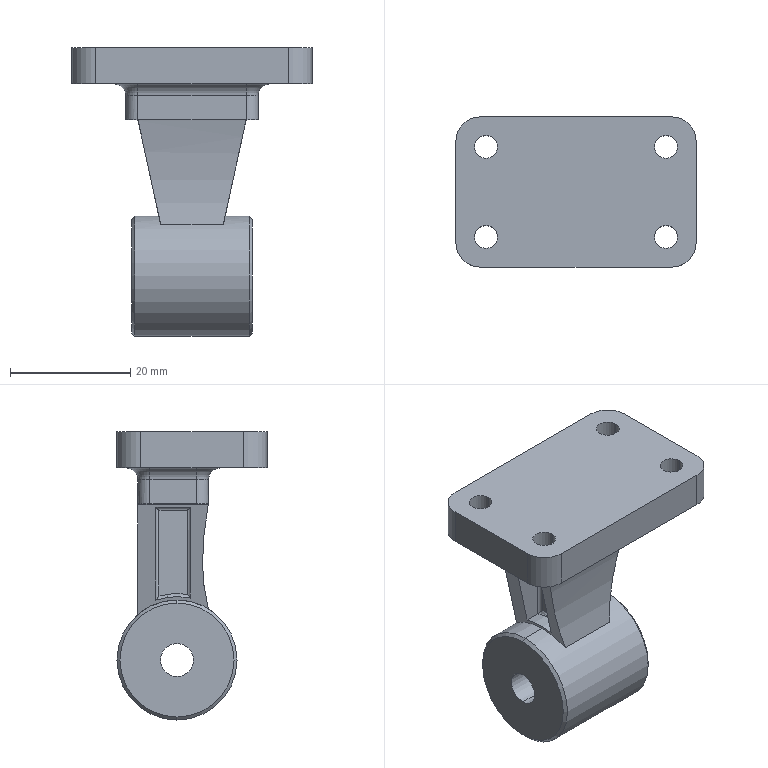Part | SolidWorks | features ICE 8, Fillet 3, Chamfer 2, Extrusion 1 | 1 solid | 76 faces | box 40 x 25 x 48 mm | volume 13548 mm3 | cylinder 37 | plane 25 | torus 7 | cone 6 | spline 1 | commonest cylinder face diameters 3.8 x8 4 x8 1 x6 8 x4 21.131 x3 0.4 x2